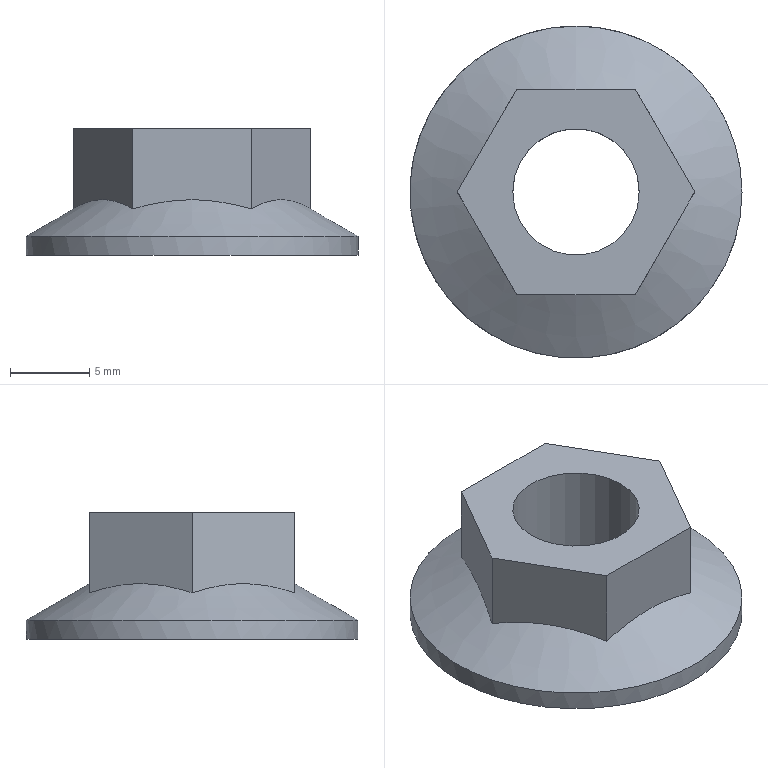Part | STEP file | 1_22 | 1 solid | 11 faces | box 21 x 21 x 8 mm | volume 1207 mm3 | plane 8 | cylinder 2 | cone 1 | commonest cylinder face diameters 8 x1 21 x1
STEP:
#1=CARTESIAN_POINT('',(0.,0.,0.));
#2=DIRECTION('',(0.,0.,1.));
#3=DIRECTION('',(1.,0.,0.));
#4=AXIS2_PLACEMENT_3D('',#1,#2,#3);
#5=CARTESIAN_POINT('',(3.753,6.5,2.929));
#6=VERTEX_POINT('',#5);
#7=CARTESIAN_POINT('',(0.,6.5,3.509));
#8=VERTEX_POINT('',#7);
#9=CARTESIAN_POINT('',(10.362,6.5,0.2));
#10=CARTESIAN_POINT('',(0.,6.5,5.268));
#11=CARTESIAN_POINT('',(-10.362,6.5,0.2));
#12=(BOUNDED_CURVE()B_SPLINE_CURVE(2,(#9,#10,#11),.UNSPECIFIED.,.F.,.F.)B_SPLINE_CURVE_WITH_KNOTS((3,3),(0.,2.176),.PIECEWISE_BEZIER_KNOTS.)CURVE()GEOMETRIC_REPRESENTATION_ITEM()RATIONAL_B_SPLINE_CURVE((1.,1.882,1.))REPRESENTATION_ITEM(''));
#13=CARTESIAN_POINT('',(0.,0.,6.262));
#14=DIRECTION('',(0.,0.,-1.));
#15=DIRECTION('',(0.,1.,0.));
#16=AXIS2_PLACEMENT_3D('',#13,#14,#15);
#17=CONICAL_SURFACE('',#16,1.732,1.047);
#18=CARTESIAN_POINT('',(0.5236,3.333));
#19=CARTESIAN_POINT('',(0.516,3.314));
#20=CARTESIAN_POINT('',(0.5008,3.278));
#21=CARTESIAN_POINT('',(0.4779,3.226));
#22=CARTESIAN_POINT('',(0.4548,3.177));
#23=CARTESIAN_POINT('',(0.4317,3.131));
#24=CARTESIAN_POINT('',(0.4084,3.088));
#25=CARTESIAN_POINT('',(0.3849,3.049));
#26=CARTESIAN_POINT('',(0.3614,3.011));
#27=CARTESIAN_POINT('',(0.3378,2.977));
#28=CARTESIAN_POINT('',(0.3141,2.945));
#29=CARTESIAN_POINT('',(0.2903,2.916));
#30=CARTESIAN_POINT('',(0.2664,2.89));
#31=CARTESIAN_POINT('',(0.2424,2.865));
#32=CARTESIAN_POINT('',(0.2184,2.844));
#33=CARTESIAN_POINT('',(0.1943,2.824));
#34=CARTESIAN_POINT('',(0.1701,2.807));
#35=CARTESIAN_POINT('',(0.1459,2.793));
#36=CARTESIAN_POINT('',(0.1217,2.78));
#37=CARTESIAN_POINT('',(0.09736,2.77));
#38=CARTESIAN_POINT('',(0.07305,2.762));
#39=CARTESIAN_POINT('',(0.04871,2.757));
#40=CARTESIAN_POINT('',(0.02436,2.754));
#41=CARTESIAN_POINT('',(0.00812,2.753));
#42=CARTESIAN_POINT('',(0.,2.753));
#43=B_SPLINE_CURVE_WITH_KNOTS('',3,(#18,#19,#20,#21,#22,#23,#24,#25,#26,#27,#28,#29,#30,#31,#32,#33,#34,#35,#36,#37,#38,#39,#40,#41,#42),.UNSPECIFIED.,.F.,.F.,(4,1,1,1,1,1,1,1,1,1,1,1,1,1,1,1,1,1,1,1,1,1,4),(0.5609,0.5848,0.6088,0.6327,0.6567,0.6806,0.7046,0.7285,0.7525,0.7764,0.8004,0.8243,0.8483,0.8722,0.8962,0.9201,0.9441,0.968,0.992,1.016,1.04,1.064,1.088),.QUASI_UNIFORM_KNOTS.);
#44=(GEOMETRIC_REPRESENTATION_CONTEXT(2)PARAMETRIC_REPRESENTATION_CONTEXT()REPRESENTATION_CONTEXT('',''));
#45=DEFINITIONAL_REPRESENTATION('',(#43),#44);
#46=PCURVE('',#17,#45);
#47=CARTESIAN_POINT('',(-4.128,6.5,8.254));
#48=DIRECTION('',(0.,1.,0.));
#49=DIRECTION('',(0.,0.,1.));
#50=AXIS2_PLACEMENT_3D('',#47,#48,#49);
#51=PLANE('',#50);
#52=CARTESIAN_POINT('',(-8.054,14.49));
#53=CARTESIAN_POINT('',(-2.986,4.128));
#54=CARTESIAN_POINT('',(-8.054,-6.234));
#55=(BOUNDED_CURVE()B_SPLINE_CURVE(2,(#52,#53,#54),.UNSPECIFIED.,.F.,.F.)B_SPLINE_CURVE_WITH_KNOTS((3,3),(0.,2.176),.PIECEWISE_BEZIER_KNOTS.)CURVE()GEOMETRIC_REPRESENTATION_ITEM()RATIONAL_B_SPLINE_CURVE((1.,1.882,1.))REPRESENTATION_ITEM(''));
#56=(GEOMETRIC_REPRESENTATION_CONTEXT(2)PARAMETRIC_REPRESENTATION_CONTEXT()REPRESENTATION_CONTEXT('',''));
#57=DEFINITIONAL_REPRESENTATION('',(#55),#56);
#58=PCURVE('',#51,#57);
#59=SURFACE_CURVE('',#12,(#46,#58),.PCURVE_S1.);
#60=EDGE_CURVE('',#6,#8,#59,.T.);
#61=ORIENTED_EDGE('',*,*,#60,.F.);
#62=CARTESIAN_POINT('',(7.506,0.,2.929));
#63=VERTEX_POINT('',#62);
#64=CARTESIAN_POINT('',(10.81,-5.724,0.2));
#65=CARTESIAN_POINT('',(5.629,3.25,5.268));
#66=CARTESIAN_POINT('',(0.4481,12.224,0.2));
#67=(BOUNDED_CURVE()B_SPLINE_CURVE(2,(#64,#65,#66),.UNSPECIFIED.,.F.,.F.)B_SPLINE_CURVE_WITH_KNOTS((3,3),(0.,2.176),.PIECEWISE_BEZIER_KNOTS.)CURVE()GEOMETRIC_REPRESENTATION_ITEM()RATIONAL_B_SPLINE_CURVE((1.,1.882,1.))REPRESENTATION_ITEM(''));
#68=CARTESIAN_POINT('',(1.571,3.333));
#69=CARTESIAN_POINT('',(1.556,3.295));
#70=CARTESIAN_POINT('',(1.525,3.224));
#71=CARTESIAN_POINT('',(1.479,3.13));
#72=CARTESIAN_POINT('',(1.432,3.047));
#73=CARTESIAN_POINT('',(1.385,2.976));
#74=CARTESIAN_POINT('',(1.338,2.915));
#75=CARTESIAN_POINT('',(1.29,2.864));
#76=CARTESIAN_POINT('',(1.241,2.823));
#77=CARTESIAN_POINT('',(1.193,2.792));
#78=CARTESIAN_POINT('',(1.145,2.769));
#79=CARTESIAN_POINT('',(1.096,2.756));
#80=CARTESIAN_POINT('',(1.047,2.751));
#81=CARTESIAN_POINT('',(0.9985,2.756));
#82=CARTESIAN_POINT('',(0.9498,2.769));
#83=CARTESIAN_POINT('',(0.9013,2.792));
#84=CARTESIAN_POINT('',(0.8529,2.823));
#85=CARTESIAN_POINT('',(0.8048,2.864));
#86=CARTESIAN_POINT('',(0.7569,2.915));
#87=CARTESIAN_POINT('',(0.7094,2.976));
#88=CARTESIAN_POINT('',(0.6622,3.047));
#89=CARTESIAN_POINT('',(0.6155,3.13));
#90=CARTESIAN_POINT('',(0.5692,3.224));
#91=CARTESIAN_POINT('',(0.5388,3.295));
#92=CARTESIAN_POINT('',(0.5236,3.333));
#93=B_SPLINE_CURVE_WITH_KNOTS('',3,(#68,#69,#70,#71,#72,#73,#74,#75,#76,#77,#78,#79,#80,#81,#82,#83,#84,#85,#86,#87,#88,#89,#90,#91,#92),.UNSPECIFIED.,.F.,.F.,(4,1,1,1,1,1,1,1,1,1,1,1,1,1,1,1,1,1,1,1,1,1,4),(0.5609,0.6088,0.6567,0.7046,0.7525,0.8004,0.8483,0.8962,0.9441,0.992,1.04,1.088,1.136,1.184,1.231,1.279,1.327,1.375,1.423,1.471,1.519,1.567,1.615),.QUASI_UNIFORM_KNOTS.);
#94=(GEOMETRIC_REPRESENTATION_CONTEXT(2)PARAMETRIC_REPRESENTATION_CONTEXT()REPRESENTATION_CONTEXT('',''));
#95=DEFINITIONAL_REPRESENTATION('',(#93),#94);
#96=PCURVE('',#17,#95);
#97=CARTESIAN_POINT('',(3.565,6.825,8.254));
#98=DIRECTION('',(0.866,0.5,0.));
#99=DIRECTION('',(0.,0.,-1.));
#100=AXIS2_PLACEMENT_3D('',#97,#98,#99);
#101=PLANE('',#100);
#102=CARTESIAN_POINT('',(8.054,-14.49));
#103=CARTESIAN_POINT('',(2.986,-4.128));
#104=CARTESIAN_POINT('',(8.054,6.234));
#105=(BOUNDED_CURVE()B_SPLINE_CURVE(2,(#102,#103,#104),.UNSPECIFIED.,.F.,.F.)B_SPLINE_CURVE_WITH_KNOTS((3,3),(0.,2.176),.PIECEWISE_BEZIER_KNOTS.)CURVE()GEOMETRIC_REPRESENTATION_ITEM()RATIONAL_B_SPLINE_CURVE((1.,1.882,1.))REPRESENTATION_ITEM(''));
#106=(GEOMETRIC_REPRESENTATION_CONTEXT(2)PARAMETRIC_REPRESENTATION_CONTEXT()REPRESENTATION_CONTEXT('',''));
#107=DEFINITIONAL_REPRESENTATION('',(#105),#106);
#108=PCURVE('',#101,#107);
#109=SURFACE_CURVE('',#67,(#96,#108),.PCURVE_S1.);
#110=EDGE_CURVE('',#63,#6,#109,.T.);
#111=ORIENTED_EDGE('',*,*,#110,.F.);
#112=CARTESIAN_POINT('',(3.753,-6.5,2.929));
#113=VERTEX_POINT('',#112);
#114=CARTESIAN_POINT('',(0.4481,-12.224,0.2));
#115=CARTESIAN_POINT('',(5.629,-3.25,5.268));
#116=CARTESIAN_POINT('',(10.81,5.724,0.2));
#117=(BOUNDED_CURVE()B_SPLINE_CURVE(2,(#114,#115,#116),.UNSPECIFIED.,.F.,.F.)B_SPLINE_CURVE_WITH_KNOTS((3,3),(0.,2.176),.PIECEWISE_BEZIER_KNOTS.)CURVE()GEOMETRIC_REPRESENTATION_ITEM()RATIONAL_B_SPLINE_CURVE((1.,1.882,1.))REPRESENTATION_ITEM(''));
#118=CARTESIAN_POINT('',(2.618,3.333));
#119=CARTESIAN_POINT('',(2.603,3.295));
#120=CARTESIAN_POINT('',(2.572,3.224));
#121=CARTESIAN_POINT('',(2.526,3.13));
#122=CARTESIAN_POINT('',(2.479,3.047));
#123=CARTESIAN_POINT('',(2.432,2.976));
#124=CARTESIAN_POINT('',(2.385,2.915));
#125=CARTESIAN_POINT('',(2.337,2.864));
#126=CARTESIAN_POINT('',(2.289,2.823));
#127=CARTESIAN_POINT('',(2.24,2.792));
#128=CARTESIAN_POINT('',(2.192,2.769));
#129=CARTESIAN_POINT('',(2.143,2.756));
#130=CARTESIAN_POINT('',(2.094,2.751));
#131=CARTESIAN_POINT('',(2.046,2.756));
#132=CARTESIAN_POINT('',(1.997,2.769));
#133=CARTESIAN_POINT('',(1.948,2.792));
#134=CARTESIAN_POINT('',(1.9,2.823));
#135=CARTESIAN_POINT('',(1.852,2.864));
#136=CARTESIAN_POINT('',(1.804,2.915));
#137=CARTESIAN_POINT('',(1.757,2.976));
#138=CARTESIAN_POINT('',(1.709,3.047));
#139=CARTESIAN_POINT('',(1.663,3.13));
#140=CARTESIAN_POINT('',(1.616,3.224));
#141=CARTESIAN_POINT('',(1.586,3.295));
#142=CARTESIAN_POINT('',(1.571,3.333));
#143=B_SPLINE_CURVE_WITH_KNOTS('',3,(#118,#119,#120,#121,#122,#123,#124,#125,#126,#127,#128,#129,#130,#131,#132,#133,#134,#135,#136,#137,#138,#139,#140,#141,#142),.UNSPECIFIED.,.F.,.F.,(4,1,1,1,1,1,1,1,1,1,1,1,1,1,1,1,1,1,1,1,1,1,4),(0.5609,0.6088,0.6567,0.7046,0.7525,0.8004,0.8483,0.8962,0.9441,0.992,1.04,1.088,1.136,1.184,1.231,1.279,1.327,1.375,1.423,1.471,1.519,1.567,1.615),.QUASI_UNIFORM_KNOTS.);
#144=(GEOMETRIC_REPRESENTATION_CONTEXT(2)PARAMETRIC_REPRESENTATION_CONTEXT()REPRESENTATION_CONTEXT('',''));
#145=DEFINITIONAL_REPRESENTATION('',(#143),#144);
#146=PCURVE('',#17,#145);
#147=CARTESIAN_POINT('',(7.693,0.325,8.254));
#148=DIRECTION('',(0.866,-0.5,0.));
#149=DIRECTION('',(0.,0.,-1.));
#150=AXIS2_PLACEMENT_3D('',#147,#148,#149);
#151=PLANE('',#150);
#152=CARTESIAN_POINT('',(8.054,-14.49));
#153=CARTESIAN_POINT('',(2.986,-4.128));
#154=CARTESIAN_POINT('',(8.054,6.234));
#155=(BOUNDED_CURVE()B_SPLINE_CURVE(2,(#152,#153,#154),.UNSPECIFIED.,.F.,.F.)B_SPLINE_CURVE_WITH_KNOTS((3,3),(0.,2.176),.PIECEWISE_BEZIER_KNOTS.)CURVE()GEOMETRIC_REPRESENTATION_ITEM()RATIONAL_B_SPLINE_CURVE((1.,1.882,1.))REPRESENTATION_ITEM(''));
#156=(GEOMETRIC_REPRESENTATION_CONTEXT(2)PARAMETRIC_REPRESENTATION_CONTEXT()REPRESENTATION_CONTEXT('',''));
#157=DEFINITIONAL_REPRESENTATION('',(#155),#156);
#158=PCURVE('',#151,#157);
#159=SURFACE_CURVE('',#117,(#146,#158),.PCURVE_S1.);
#160=EDGE_CURVE('',#113,#63,#159,.T.);
#161=ORIENTED_EDGE('',*,*,#160,.F.);
#162=CARTESIAN_POINT('',(0.,-6.5,3.509));
#163=VERTEX_POINT('',#162);
#164=CARTESIAN_POINT('',(-10.362,-6.5,0.2));
#165=CARTESIAN_POINT('',(0.,-6.5,5.268));
#166=CARTESIAN_POINT('',(10.362,-6.5,0.2));
#167=(BOUNDED_CURVE()B_SPLINE_CURVE(2,(#164,#165,#166),.UNSPECIFIED.,.F.,.F.)B_SPLINE_CURVE_WITH_KNOTS((3,3),(0.,2.176),.PIECEWISE_BEZIER_KNOTS.)CURVE()GEOMETRIC_REPRESENTATION_ITEM()RATIONAL_B_SPLINE_CURVE((1.,1.882,1.))REPRESENTATION_ITEM(''));
#168=CARTESIAN_POINT('',(3.142,2.753));
#169=CARTESIAN_POINT('',(3.133,2.753));
#170=CARTESIAN_POINT('',(3.117,2.754));
#171=CARTESIAN_POINT('',(3.093,2.757));
#172=CARTESIAN_POINT('',(3.069,2.762));
#173=CARTESIAN_POINT('',(3.044,2.77));
#174=CARTESIAN_POINT('',(3.02,2.78));
#175=CARTESIAN_POINT('',(2.996,2.793));
#176=CARTESIAN_POINT('',(2.971,2.807));
#177=CARTESIAN_POINT('',(2.947,2.824));
#178=CARTESIAN_POINT('',(2.923,2.844));
#179=CARTESIAN_POINT('',(2.899,2.865));
#180=CARTESIAN_POINT('',(2.875,2.89));
#181=CARTESIAN_POINT('',(2.851,2.916));
#182=CARTESIAN_POINT('',(2.828,2.945));
#183=CARTESIAN_POINT('',(2.804,2.977));
#184=CARTESIAN_POINT('',(2.78,3.011));
#185=CARTESIAN_POINT('',(2.757,3.049));
#186=CARTESIAN_POINT('',(2.733,3.088));
#187=CARTESIAN_POINT('',(2.71,3.131));
#188=CARTESIAN_POINT('',(2.687,3.177));
#189=CARTESIAN_POINT('',(2.664,3.226));
#190=CARTESIAN_POINT('',(2.641,3.278));
#191=CARTESIAN_POINT('',(2.626,3.314));
#192=CARTESIAN_POINT('',(2.618,3.333));
#193=B_SPLINE_CURVE_WITH_KNOTS('',3,(#168,#169,#170,#171,#172,#173,#174,#175,#176,#177,#178,#179,#180,#181,#182,#183,#184,#185,#186,#187,#188,#189,#190,#191,#192),.UNSPECIFIED.,.F.,.F.,(4,1,1,1,1,1,1,1,1,1,1,1,1,1,1,1,1,1,1,1,1,1,4),(1.088,1.112,1.136,1.16,1.184,1.208,1.231,1.255,1.279,1.303,1.327,1.351,1.375,1.399,1.423,1.447,1.471,1.495,1.519,1.543,1.567,1.591,1.615),.QUASI_UNIFORM_KNOTS.);
#194=(GEOMETRIC_REPRESENTATION_CONTEXT(2)PARAMETRIC_REPRESENTATION_CONTEXT()REPRESENTATION_CONTEXT('',''));
#195=DEFINITIONAL_REPRESENTATION('',(#193),#194);
#196=PCURVE('',#17,#195);
#197=CARTESIAN_POINT('',(4.128,-6.5,8.254));
#198=DIRECTION('',(0.,-1.,0.));
#199=DIRECTION('',(0.,0.,-1.));
#200=AXIS2_PLACEMENT_3D('',#197,#198,#199);
#201=PLANE('',#200);
#202=CARTESIAN_POINT('',(8.054,-14.49));
#203=CARTESIAN_POINT('',(2.986,-4.128));
#204=CARTESIAN_POINT('',(8.054,6.234));
#205=(BOUNDED_CURVE()B_SPLINE_CURVE(2,(#202,#203,#204),.UNSPECIFIED.,.F.,.F.)B_SPLINE_CURVE_WITH_KNOTS((3,3),(0.,2.176),.PIECEWISE_BEZIER_KNOTS.)CURVE()GEOMETRIC_REPRESENTATION_ITEM()RATIONAL_B_SPLINE_CURVE((1.,1.882,1.))REPRESENTATION_ITEM(''));
#206=(GEOMETRIC_REPRESENTATION_CONTEXT(2)PARAMETRIC_REPRESENTATION_CONTEXT()REPRESENTATION_CONTEXT('',''));
#207=DEFINITIONAL_REPRESENTATION('',(#205),#206);
#208=PCURVE('',#201,#207);
#209=SURFACE_CURVE('',#167,(#196,#208),.PCURVE_S1.);
#210=EDGE_CURVE('',#163,#113,#209,.T.);
#211=ORIENTED_EDGE('',*,*,#210,.F.);
#212=CARTESIAN_POINT('',(-3.753,-6.5,2.929));
#213=VERTEX_POINT('',#212);
#214=CARTESIAN_POINT('',(-10.362,-6.5,0.2));
#215=CARTESIAN_POINT('',(0.,-6.5,5.268));
#216=CARTESIAN_POINT('',(10.362,-6.5,0.2));
#217=(BOUNDED_CURVE()B_SPLINE_CURVE(2,(#214,#215,#216),.UNSPECIFIED.,.F.,.F.)B_SPLINE_CURVE_WITH_KNOTS((3,3),(0.,2.176),.PIECEWISE_BEZIER_KNOTS.)CURVE()GEOMETRIC_REPRESENTATION_ITEM()RATIONAL_B_SPLINE_CURVE((1.,1.882,1.))REPRESENTATION_ITEM(''));
#218=CARTESIAN_POINT('',(3.665,3.333));
#219=CARTESIAN_POINT('',(3.658,3.314));
#220=CARTESIAN_POINT('',(3.642,3.278));
#221=CARTESIAN_POINT('',(3.619,3.226));
#222=CARTESIAN_POINT('',(3.596,3.177));
#223=CARTESIAN_POINT('',(3.573,3.131));
#224=CARTESIAN_POINT('',(3.55,3.088));
#225=CARTESIAN_POINT('',(3.527,3.049));
#226=CARTESIAN_POINT('',(3.503,3.011));
#227=CARTESIAN_POINT('',(3.479,2.977));
#228=CARTESIAN_POINT('',(3.456,2.945));
#229=CARTESIAN_POINT('',(3.432,2.916));
#230=CARTESIAN_POINT('',(3.408,2.89));
#231=CARTESIAN_POINT('',(3.384,2.865));
#232=CARTESIAN_POINT('',(3.36,2.844));
#233=CARTESIAN_POINT('',(3.336,2.824));
#234=CARTESIAN_POINT('',(3.312,2.807));
#235=CARTESIAN_POINT('',(3.287,2.793));
#236=CARTESIAN_POINT('',(3.263,2.78));
#237=CARTESIAN_POINT('',(3.239,2.77));
#238=CARTESIAN_POINT('',(3.215,2.762));
#239=CARTESIAN_POINT('',(3.19,2.757));
#240=CARTESIAN_POINT('',(3.166,2.754));
#241=CARTESIAN_POINT('',(3.15,2.753));
#242=CARTESIAN_POINT('',(3.142,2.753));
#243=B_SPLINE_CURVE_WITH_KNOTS('',3,(#218,#219,#220,#221,#222,#223,#224,#225,#226,#227,#228,#229,#230,#231,#232,#233,#234,#235,#236,#237,#238,#239,#240,#241,#242),.UNSPECIFIED.,.F.,.F.,(4,1,1,1,1,1,1,1,1,1,1,1,1,1,1,1,1,1,1,1,1,1,4),(0.5609,0.5848,0.6088,0.6327,0.6567,0.6806,0.7046,0.7285,0.7525,0.7764,0.8004,0.8243,0.8483,0.8722,0.8962,0.9201,0.9441,0.968,0.992,1.016,1.04,1.064,1.088),.QUASI_UNIFORM_KNOTS.);
#244=(GEOMETRIC_REPRESENTATION_CONTEXT(2)PARAMETRIC_REPRESENTATION_CONTEXT()REPRESENTATION_CONTEXT('',''));
#245=DEFINITIONAL_REPRESENTATION('',(#243),#244);
#246=PCURVE('',#17,#245);
#247=CARTESIAN_POINT('',(8.054,-14.49));
#248=CARTESIAN_POINT('',(2.986,-4.128));
#249=CARTESIAN_POINT('',(8.054,6.234));
#250=(BOUNDED_CURVE()B_SPLINE_CURVE(2,(#247,#248,#249),.UNSPECIFIED.,.F.,.F.)B_SPLINE_CURVE_WITH_KNOTS((3,3),(0.,2.176),.PIECEWISE_BEZIER_KNOTS.)CURVE()GEOMETRIC_REPRESENTATION_ITEM()RATIONAL_B_SPLINE_CURVE((1.,1.882,1.))REPRESENTATION_ITEM(''));
#251=(GEOMETRIC_REPRESENTATION_CONTEXT(2)PARAMETRIC_REPRESENTATION_CONTEXT()REPRESENTATION_CONTEXT('',''));
#252=DEFINITIONAL_REPRESENTATION('',(#250),#251);
#253=PCURVE('',#201,#252);
#254=SURFACE_CURVE('',#217,(#246,#253),.PCURVE_S1.);
#255=EDGE_CURVE('',#213,#163,#254,.T.);
#256=ORIENTED_EDGE('',*,*,#255,.F.);
#257=CARTESIAN_POINT('',(-7.506,0.,2.929));
#258=VERTEX_POINT('',#257);
#259=CARTESIAN_POINT('',(-10.81,5.724,0.2));
#260=CARTESIAN_POINT('',(-5.629,-3.25,5.268));
#261=CARTESIAN_POINT('',(-0.4481,-12.224,0.2));
#262=(BOUNDED_CURVE()B_SPLINE_CURVE(2,(#259,#260,#261),.UNSPECIFIED.,.F.,.F.)B_SPLINE_CURVE_WITH_KNOTS((3,3),(0.,2.176),.PIECEWISE_BEZIER_KNOTS.)CURVE()GEOMETRIC_REPRESENTATION_ITEM()RATIONAL_B_SPLINE_CURVE((1.,1.882,1.))REPRESENTATION_ITEM(''));
#263=CARTESIAN_POINT('',(4.712,3.333));
#264=CARTESIAN_POINT('',(4.697,3.295));
#265=CARTESIAN_POINT('',(4.667,3.224));
#266=CARTESIAN_POINT('',(4.621,3.13));
#267=CARTESIAN_POINT('',(4.574,3.047));
#268=CARTESIAN_POINT('',(4.527,2.976));
#269=CARTESIAN_POINT('',(4.479,2.915));
#270=CARTESIAN_POINT('',(4.431,2.864));
#271=CARTESIAN_POINT('',(4.383,2.823));
#272=CARTESIAN_POINT('',(4.335,2.792));
#273=CARTESIAN_POINT('',(4.286,2.769));
#274=CARTESIAN_POINT('',(4.238,2.756));
#275=CARTESIAN_POINT('',(4.189,2.751));
#276=CARTESIAN_POINT('',(4.14,2.756));
#277=CARTESIAN_POINT('',(4.091,2.769));
#278=CARTESIAN_POINT('',(4.043,2.792));
#279=CARTESIAN_POINT('',(3.994,2.823));
#280=CARTESIAN_POINT('',(3.946,2.864));
#281=CARTESIAN_POINT('',(3.898,2.915));
#282=CARTESIAN_POINT('',(3.851,2.976));
#283=CARTESIAN_POINT('',(3.804,3.047));
#284=CARTESIAN_POINT('',(3.757,3.13));
#285=CARTESIAN_POINT('',(3.711,3.224));
#286=CARTESIAN_POINT('',(3.68,3.295));
#287=CARTESIAN_POINT('',(3.665,3.333));
#288=B_SPLINE_CURVE_WITH_KNOTS('',3,(#263,#264,#265,#266,#267,#268,#269,#270,#271,#272,#273,#274,#275,#276,#277,#278,#279,#280,#281,#282,#283,#284,#285,#286,#287),.UNSPECIFIED.,.F.,.F.,(4,1,1,1,1,1,1,1,1,1,1,1,1,1,1,1,1,1,1,1,1,1,4),(0.5609,0.6088,0.6567,0.7046,0.7525,0.8004,0.8483,0.8962,0.9441,0.992,1.04,1.088,1.136,1.184,1.231,1.279,1.327,1.375,1.423,1.471,1.519,1.567,1.615),.QUASI_UNIFORM_KNOTS.);
#289=(GEOMETRIC_REPRESENTATION_CONTEXT(2)PARAMETRIC_REPRESENTATION_CONTEXT()REPRESENTATION_CONTEXT('',''));
#290=DEFINITIONAL_REPRESENTATION('',(#288),#289);
#291=PCURVE('',#17,#290);
#292=CARTESIAN_POINT('',(-3.565,-6.825,8.254));
#293=DIRECTION('',(-0.866,-0.5,0.));
#294=DIRECTION('',(0.,0.,1.));
#295=AXIS2_PLACEMENT_3D('',#292,#293,#294);
#296=PLANE('',#295);
#297=CARTESIAN_POINT('',(-8.054,14.49));
#298=CARTESIAN_POINT('',(-2.986,4.128));
#299=CARTESIAN_POINT('',(-8.054,-6.234));
#300=(BOUNDED_CURVE()B_SPLINE_CURVE(2,(#297,#298,#299),.UNSPECIFIED.,.F.,.F.)B_SPLINE_CURVE_WITH_KNOTS((3,3),(0.,2.176),.PIECEWISE_BEZIER_KNOTS.)CURVE()GEOMETRIC_REPRESENTATION_ITEM()RATIONAL_B_SPLINE_CURVE((1.,1.882,1.))REPRESENTATION_ITEM(''));
#301=(GEOMETRIC_REPRESENTATION_CONTEXT(2)PARAMETRIC_REPRESENTATION_CONTEXT()REPRESENTATION_CONTEXT('',''));
#302=DEFINITIONAL_REPRESENTATION('',(#300),#301);
#303=PCURVE('',#296,#302);
#304=SURFACE_CURVE('',#262,(#291,#303),.PCURVE_S1.);
#305=EDGE_CURVE('',#258,#213,#304,.T.);
#306=ORIENTED_EDGE('',*,*,#305,.F.);
#307=CARTESIAN_POINT('',(-3.753,6.5,2.929));
#308=VERTEX_POINT('',#307);
#309=CARTESIAN_POINT('',(-0.4481,12.224,0.2));
#310=CARTESIAN_POINT('',(-5.629,3.25,5.268));
#311=CARTESIAN_POINT('',(-10.81,-5.724,0.2));
#312=(BOUNDED_CURVE()B_SPLINE_CURVE(2,(#309,#310,#311),.UNSPECIFIED.,.F.,.F.)B_SPLINE_CURVE_WITH_KNOTS((3,3),(0.,2.176),.PIECEWISE_BEZIER_KNOTS.)CURVE()GEOMETRIC_REPRESENTATION_ITEM()RATIONAL_B_SPLINE_CURVE((1.,1.882,1.))REPRESENTATION_ITEM(''));
#313=CARTESIAN_POINT('',(5.76,3.333));
#314=CARTESIAN_POINT('',(5.744,3.295));
#315=CARTESIAN_POINT('',(5.714,3.224));
#316=CARTESIAN_POINT('',(5.668,3.13));
#317=CARTESIAN_POINT('',(5.621,3.047));
#318=CARTESIAN_POINT('',(5.574,2.976));
#319=CARTESIAN_POINT('',(5.526,2.915));
#320=CARTESIAN_POINT('',(5.478,2.864));
#321=CARTESIAN_POINT('',(5.43,2.823));
#322=CARTESIAN_POINT('',(5.382,2.792));
#323=CARTESIAN_POINT('',(5.333,2.769));
#324=CARTESIAN_POINT('',(5.285,2.756));
#325=CARTESIAN_POINT('',(5.236,2.751));
#326=CARTESIAN_POINT('',(5.187,2.756));
#327=CARTESIAN_POINT('',(5.139,2.769));
#328=CARTESIAN_POINT('',(5.09,2.792));
#329=CARTESIAN_POINT('',(5.042,2.823));
#330=CARTESIAN_POINT('',(4.994,2.864));
#331=CARTESIAN_POINT('',(4.946,2.915));
#332=CARTESIAN_POINT('',(4.898,2.976));
#333=CARTESIAN_POINT('',(4.851,3.047));
#334=CARTESIAN_POINT('',(4.804,3.13));
#335=CARTESIAN_POINT('',(4.758,3.224));
#336=CARTESIAN_POINT('',(4.728,3.295));
#337=CARTESIAN_POINT('',(4.712,3.333));
#338=B_SPLINE_CURVE_WITH_KNOTS('',3,(#313,#314,#315,#316,#317,#318,#319,#320,#321,#322,#323,#324,#325,#326,#327,#328,#329,#330,#331,#332,#333,#334,#335,#336,#337),.UNSPECIFIED.,.F.,.F.,(4,1,1,1,1,1,1,1,1,1,1,1,1,1,1,1,1,1,1,1,1,1,4),(0.5609,0.6088,0.6567,0.7046,0.7525,0.8004,0.8483,0.8962,0.9441,0.992,1.04,1.088,1.136,1.184,1.231,1.279,1.327,1.375,1.423,1.471,1.519,1.567,1.615),.QUASI_UNIFORM_KNOTS.);
#339=(GEOMETRIC_REPRESENTATION_CONTEXT(2)PARAMETRIC_REPRESENTATION_CONTEXT()REPRESENTATION_CONTEXT('',''));
#340=DEFINITIONAL_REPRESENTATION('',(#338),#339);
#341=PCURVE('',#17,#340);
#342=CARTESIAN_POINT('',(-7.693,-0.325,8.254));
#343=DIRECTION('',(-0.866,0.5,0.));
#344=DIRECTION('',(0.,0.,1.));
#345=AXIS2_PLACEMENT_3D('',#342,#343,#344);
#346=PLANE('',#345);
#347=CARTESIAN_POINT('',(-8.054,14.49));
#348=CARTESIAN_POINT('',(-2.986,4.128));
#349=CARTESIAN_POINT('',(-8.054,-6.234));
#350=(BOUNDED_CURVE()B_SPLINE_CURVE(2,(#347,#348,#349),.UNSPECIFIED.,.F.,.F.)B_SPLINE_CURVE_WITH_KNOTS((3,3),(0.,2.176),.PIECEWISE_BEZIER_KNOTS.)CURVE()GEOMETRIC_REPRESENTATION_ITEM()RATIONAL_B_SPLINE_CURVE((1.,1.882,1.))REPRESENTATION_ITEM(''));
#351=(GEOMETRIC_REPRESENTATION_CONTEXT(2)PARAMETRIC_REPRESENTATION_CONTEXT()REPRESENTATION_CONTEXT('',''));
#352=DEFINITIONAL_REPRESENTATION('',(#350),#351);
#353=PCURVE('',#346,#352);
#354=SURFACE_CURVE('',#312,(#341,#353),.PCURVE_S1.);
#355=EDGE_CURVE('',#308,#258,#354,.T.);
#356=ORIENTED_EDGE('',*,*,#355,.F.);
#357=CARTESIAN_POINT('',(10.362,6.5,0.2));
#358=CARTESIAN_POINT('',(0.,6.5,5.268));
#359=CARTESIAN_POINT('',(-10.362,6.5,0.2));
#360=(BOUNDED_CURVE()B_SPLINE_CURVE(2,(#357,#358,#359),.UNSPECIFIED.,.F.,.F.)B_SPLINE_CURVE_WITH_KNOTS((3,3),(0.,2.176),.PIECEWISE_BEZIER_KNOTS.)CURVE()GEOMETRIC_REPRESENTATION_ITEM()RATIONAL_B_SPLINE_CURVE((1.,1.882,1.))REPRESENTATION_ITEM(''));
#361=CARTESIAN_POINT('',(6.283,2.753));
#362=CARTESIAN_POINT('',(6.275,2.753));
#363=CARTESIAN_POINT('',(6.259,2.754));
#364=CARTESIAN_POINT('',(6.234,2.757));
#365=CARTESIAN_POINT('',(6.21,2.762));
#366=CARTESIAN_POINT('',(6.186,2.77));
#367=CARTESIAN_POINT('',(6.162,2.78));
#368=CARTESIAN_POINT('',(6.137,2.793));
#369=CARTESIAN_POINT('',(6.113,2.807));
#370=CARTESIAN_POINT('',(6.089,2.824));
#371=CARTESIAN_POINT('',(6.065,2.844));
#372=CARTESIAN_POINT('',(6.041,2.865));
#373=CARTESIAN_POINT('',(6.017,2.89));
#374=CARTESIAN_POINT('',(5.993,2.916));
#375=CARTESIAN_POINT('',(5.969,2.945));
#376=CARTESIAN_POINT('',(5.945,2.977));
#377=CARTESIAN_POINT('',(5.922,3.011));
#378=CARTESIAN_POINT('',(5.898,3.049));
#379=CARTESIAN_POINT('',(5.875,3.088));
#380=CARTESIAN_POINT('',(5.852,3.131));
#381=CARTESIAN_POINT('',(5.828,3.177));
#382=CARTESIAN_POINT('',(5.805,3.226));
#383=CARTESIAN_POINT('',(5.782,3.278));
#384=CARTESIAN_POINT('',(5.767,3.314));
#385=CARTESIAN_POINT('',(5.76,3.333));
#386=B_SPLINE_CURVE_WITH_KNOTS('',3,(#361,#362,#363,#364,#365,#366,#367,#368,#369,#370,#371,#372,#373,#374,#375,#376,#377,#378,#379,#380,#381,#382,#383,#384,#385),.UNSPECIFIED.,.F.,.F.,(4,1,1,1,1,1,1,1,1,1,1,1,1,1,1,1,1,1,1,1,1,1,4),(1.088,1.112,1.136,1.16,1.184,1.208,1.231,1.255,1.279,1.303,1.327,1.351,1.375,1.399,1.423,1.447,1.471,1.495,1.519,1.543,1.567,1.591,1.615),.QUASI_UNIFORM_KNOTS.);
#387=(GEOMETRIC_REPRESENTATION_CONTEXT(2)PARAMETRIC_REPRESENTATION_CONTEXT()REPRESENTATION_CONTEXT('',''));
#388=DEFINITIONAL_REPRESENTATION('',(#386),#387);
#389=PCURVE('',#17,#388);
#390=CARTESIAN_POINT('',(-8.054,14.49));
#391=CARTESIAN_POINT('',(-2.986,4.128));
#392=CARTESIAN_POINT('',(-8.054,-6.234));
#393=(BOUNDED_CURVE()B_SPLINE_CURVE(2,(#390,#391,#392),.UNSPECIFIED.,.F.,.F.)B_SPLINE_CURVE_WITH_KNOTS((3,3),(0.,2.176),.PIECEWISE_BEZIER_KNOTS.)CURVE()GEOMETRIC_REPRESENTATION_ITEM()RATIONAL_B_SPLINE_CURVE((1.,1.882,1.))REPRESENTATION_ITEM(''));
#394=(GEOMETRIC_REPRESENTATION_CONTEXT(2)PARAMETRIC_REPRESENTATION_CONTEXT()REPRESENTATION_CONTEXT('',''));
#395=DEFINITIONAL_REPRESENTATION('',(#393),#394);
#396=PCURVE('',#51,#395);
#397=SURFACE_CURVE('',#360,(#389,#396),.PCURVE_S1.);
#398=EDGE_CURVE('',#8,#308,#397,.T.);
#399=ORIENTED_EDGE('',*,*,#398,.F.);
#400=CARTESIAN_POINT('',(0.,10.5,1.2));
#401=VERTEX_POINT('',#400);
#402=CARTESIAN_POINT('',(0.,6.5,3.509));
#403=CARTESIAN_POINT('',(0.,10.5,1.2));
#404=B_SPLINE_CURVE_WITH_KNOTS('',1,(#402,#403),.UNSPECIFIED.,.F.,.F.,(2,2),(5.506,10.124),.PIECEWISE_BEZIER_KNOTS.);
#405=CARTESIAN_POINT('',(6.283,0.));
#406=DIRECTION('',(0.,1.));
#407=VECTOR('',#406,1.);
#408=LINE('',#405,#407);
#409=(GEOMETRIC_REPRESENTATION_CONTEXT(2)PARAMETRIC_REPRESENTATION_CONTEXT()REPRESENTATION_CONTEXT('',''));
#410=DEFINITIONAL_REPRESENTATION('',(#408),#409);
#411=PCURVE('',#17,#410);
#412=CARTESIAN_POINT('',(0.,0.));
#413=DIRECTION('',(0.,1.));
#414=VECTOR('',#413,1.);
#415=LINE('',#412,#414);
#416=(GEOMETRIC_REPRESENTATION_CONTEXT(2)PARAMETRIC_REPRESENTATION_CONTEXT()REPRESENTATION_CONTEXT('',''));
#417=DEFINITIONAL_REPRESENTATION('',(#415),#416);
#418=PCURVE('',#17,#417);
#419=SEAM_CURVE('',#404,(#411,#418),.PCURVE_S1.);
#420=EDGE_CURVE('',#8,#401,#419,.T.);
#421=ORIENTED_EDGE('',*,*,#420,.T.);
#422=CARTESIAN_POINT('',(10.5,0.,1.2));
#423=VERTEX_POINT('',#422);
#424=CARTESIAN_POINT('',(0.,0.,1.2));
#425=DIRECTION('',(0.,0.,-1.));
#426=DIRECTION('',(1.,0.,0.));
#427=AXIS2_PLACEMENT_3D('',#424,#425,#426);
#428=CIRCLE('',#427,10.5);
#429=CARTESIAN_POINT('',(-4.712,5.062));
#430=DIRECTION('',(1.,0.));
#431=VECTOR('',#430,1.);
#432=LINE('',#429,#431);
#433=(GEOMETRIC_REPRESENTATION_CONTEXT(2)PARAMETRIC_REPRESENTATION_CONTEXT()REPRESENTATION_CONTEXT('',''));
#434=DEFINITIONAL_REPRESENTATION('',(#432),#433);
#435=PCURVE('',#17,#434);
#436=CARTESIAN_POINT('',(0.,0.,8.4));
#437=DIRECTION('',(0.,0.,-1.));
#438=DIRECTION('',(1.,0.,0.));
#439=AXIS2_PLACEMENT_3D('',#436,#437,#438);
#440=CYLINDRICAL_SURFACE('',#439,10.5);
#441=CARTESIAN_POINT('',(-6.283,7.2));
#442=DIRECTION('',(1.,0.));
#443=VECTOR('',#442,1.);
#444=LINE('',#441,#443);
#445=(GEOMETRIC_REPRESENTATION_CONTEXT(2)PARAMETRIC_REPRESENTATION_CONTEXT()REPRESENTATION_CONTEXT('',''));
#446=DEFINITIONAL_REPRESENTATION('',(#444),#445);
#447=PCURVE('',#440,#446);
#448=SURFACE_CURVE('',#428,(#435,#447),.PCURVE_S1.);
#449=EDGE_CURVE('',#423,#401,#448,.T.);
#450=ORIENTED_EDGE('',*,*,#449,.F.);
#451=CARTESIAN_POINT('',(0.,0.,1.2));
#452=DIRECTION('',(0.,0.,-1.));
#453=DIRECTION('',(1.,0.,0.));
#454=AXIS2_PLACEMENT_3D('',#451,#452,#453);
#455=CIRCLE('',#454,10.5);
#456=CARTESIAN_POINT('',(-4.712,5.062));
#457=DIRECTION('',(1.,0.));
#458=VECTOR('',#457,1.);
#459=LINE('',#456,#458);
#460=(GEOMETRIC_REPRESENTATION_CONTEXT(2)PARAMETRIC_REPRESENTATION_CONTEXT()REPRESENTATION_CONTEXT('',''));
#461=DEFINITIONAL_REPRESENTATION('',(#459),#460);
#462=PCURVE('',#17,#461);
#463=CARTESIAN_POINT('',(0.,7.2));
#464=DIRECTION('',(1.,0.));
#465=VECTOR('',#464,1.);
#466=LINE('',#463,#465);
#467=(GEOMETRIC_REPRESENTATION_CONTEXT(2)PARAMETRIC_REPRESENTATION_CONTEXT()REPRESENTATION_CONTEXT('',''));
#468=DEFINITIONAL_REPRESENTATION('',(#466),#467);
#469=PCURVE('',#440,#468);
#470=SURFACE_CURVE('',#455,(#462,#469),.PCURVE_S1.);
#471=EDGE_CURVE('',#401,#423,#470,.T.);
#472=ORIENTED_EDGE('',*,*,#471,.F.);
#473=ORIENTED_EDGE('',*,*,#420,.F.);
#474=EDGE_LOOP('',(#61,#111,#161,#211,#256,#306,#356,#399,#421,#450,#472,#473));
#475=FACE_BOUND('',#474,.T.);
#476=ADVANCED_FACE('',(#475),#17,.T.);
#477=ORIENTED_EDGE('',*,*,#471,.T.);
#478=CARTESIAN_POINT('',(10.5,0.,0.));
#479=VERTEX_POINT('',#478);
#480=CARTESIAN_POINT('',(10.5,0.,1.2));
#481=CARTESIAN_POINT('',(10.5,0.,0.));
#482=B_SPLINE_CURVE_WITH_KNOTS('',1,(#480,#481),.UNSPECIFIED.,.F.,.F.,(2,2),(7.2,8.4),.PIECEWISE_BEZIER_KNOTS.);
#483=CARTESIAN_POINT('',(6.283,0.));
#484=DIRECTION('',(0.,1.));
#485=VECTOR('',#484,1.);
#486=LINE('',#483,#485);
#487=(GEOMETRIC_REPRESENTATION_CONTEXT(2)PARAMETRIC_REPRESENTATION_CONTEXT()REPRESENTATION_CONTEXT('',''));
#488=DEFINITIONAL_REPRESENTATION('',(#486),#487);
#489=PCURVE('',#440,#488);
#490=CARTESIAN_POINT('',(0.,0.));
#491=DIRECTION('',(0.,1.));
#492=VECTOR('',#491,1.);
#493=LINE('',#490,#492);
#494=(GEOMETRIC_REPRESENTATION_CONTEXT(2)PARAMETRIC_REPRESENTATION_CONTEXT()REPRESENTATION_CONTEXT('',''));
#495=DEFINITIONAL_REPRESENTATION('',(#493),#494);
#496=PCURVE('',#440,#495);
#497=SEAM_CURVE('',#482,(#489,#496),.PCURVE_S1.);
#498=EDGE_CURVE('',#423,#479,#497,.T.);
#499=ORIENTED_EDGE('',*,*,#498,.T.);
#500=CARTESIAN_POINT('',(0.,0.,0.));
#501=DIRECTION('',(0.,0.,-1.));
#502=DIRECTION('',(-1.,0.,0.));
#503=AXIS2_PLACEMENT_3D('',#500,#501,#502);
#504=CIRCLE('',#503,10.5);
#505=CARTESIAN_POINT('',(-3.142,8.4));
#506=DIRECTION('',(1.,0.));
#507=VECTOR('',#506,1.);
#508=LINE('',#505,#507);
#509=(GEOMETRIC_REPRESENTATION_CONTEXT(2)PARAMETRIC_REPRESENTATION_CONTEXT()REPRESENTATION_CONTEXT('',''));
#510=DEFINITIONAL_REPRESENTATION('',(#508),#509);
#511=PCURVE('',#440,#510);
#512=CARTESIAN_POINT('',(11.55,-11.55,0.));
#513=DIRECTION('',(0.,0.,-1.));
#514=DIRECTION('',(-1.,0.,0.));
#515=AXIS2_PLACEMENT_3D('',#512,#513,#514);
#516=PLANE('',#515);
#517=CARTESIAN_POINT('',(11.55,11.55));
#518=DIRECTION('',(1.,0.));
#519=AXIS2_PLACEMENT_2D('',#517,#518);
#520=CIRCLE('',#519,10.5);
#521=(GEOMETRIC_REPRESENTATION_CONTEXT(2)PARAMETRIC_REPRESENTATION_CONTEXT()REPRESENTATION_CONTEXT('',''));
#522=DEFINITIONAL_REPRESENTATION('',(#520),#521);
#523=PCURVE('',#516,#522);
#524=SURFACE_CURVE('',#504,(#511,#523),.PCURVE_S1.);
#525=EDGE_CURVE('',#479,#479,#524,.T.);
#526=ORIENTED_EDGE('',*,*,#525,.F.);
#527=ORIENTED_EDGE('',*,*,#498,.F.);
#528=ORIENTED_EDGE('',*,*,#449,.T.);
#529=EDGE_LOOP('',(#477,#499,#526,#527,#528));
#530=FACE_BOUND('',#529,.T.);
#531=ADVANCED_FACE('',(#530),#440,.T.);
#532=CARTESIAN_POINT('',(3.753,-6.5,8.));
#533=VERTEX_POINT('',#532);
#534=CARTESIAN_POINT('',(3.753,-6.5,8.));
#535=DIRECTION('',(0.,0.,-1.));
#536=VECTOR('',#535,1.);
#537=LINE('',#534,#536);
#538=CARTESIAN_POINT('',(0.2536,-7.881));
#539=DIRECTION('',(1.,0.));
#540=VECTOR('',#539,1.);
#541=LINE('',#538,#540);
#542=(GEOMETRIC_REPRESENTATION_CONTEXT(2)PARAMETRIC_REPRESENTATION_CONTEXT()REPRESENTATION_CONTEXT('',''));
#543=DEFINITIONAL_REPRESENTATION('',(#541),#542);
#544=PCURVE('',#151,#543);
#545=CARTESIAN_POINT('',(0.2536,-0.3753));
#546=DIRECTION('',(1.,0.));
#547=VECTOR('',#546,1.);
#548=LINE('',#545,#547);
#549=(GEOMETRIC_REPRESENTATION_CONTEXT(2)PARAMETRIC_REPRESENTATION_CONTEXT()REPRESENTATION_CONTEXT('',''));
#550=DEFINITIONAL_REPRESENTATION('',(#548),#549);
#551=PCURVE('',#201,#550);
#552=SURFACE_CURVE('',#537,(#544,#551),.PCURVE_S1.);
#553=EDGE_CURVE('',#533,#113,#552,.T.);
#554=ORIENTED_EDGE('',*,*,#553,.T.);
#555=ORIENTED_EDGE('',*,*,#160,.T.);
#556=CARTESIAN_POINT('',(7.506,0.,8.));
#557=VERTEX_POINT('',#556);
#558=CARTESIAN_POINT('',(7.506,-0.000000001,8.));
#559=DIRECTION('',(0.,0.,-1.));
#560=VECTOR('',#559,1.);
#561=LINE('',#558,#560);
#562=CARTESIAN_POINT('',(0.2536,-0.3753));
#563=DIRECTION('',(1.,0.));
#564=VECTOR('',#563,1.);
#565=LINE('',#562,#564);
#566=(GEOMETRIC_REPRESENTATION_CONTEXT(2)PARAMETRIC_REPRESENTATION_CONTEXT()REPRESENTATION_CONTEXT('',''));
#567=DEFINITIONAL_REPRESENTATION('',(#565),#566);
#568=PCURVE('',#151,#567);
#569=CARTESIAN_POINT('',(0.2536,-7.881));
#570=DIRECTION('',(1.,0.));
#571=VECTOR('',#570,1.);
#572=LINE('',#569,#571);
#573=(GEOMETRIC_REPRESENTATION_CONTEXT(2)PARAMETRIC_REPRESENTATION_CONTEXT()REPRESENTATION_CONTEXT('',''));
#574=DEFINITIONAL_REPRESENTATION('',(#572),#573);
#575=PCURVE('',#101,#574);
#576=SURFACE_CURVE('',#561,(#568,#575),.PCURVE_S1.);
#577=EDGE_CURVE('',#557,#63,#576,.T.);
#578=ORIENTED_EDGE('',*,*,#577,.F.);
#579=CARTESIAN_POINT('',(7.506,0.,8.));
#580=DIRECTION('',(-0.5,-0.866,0.));
#581=VECTOR('',#580,1.);
#582=LINE('',#579,#581);
#583=CARTESIAN_POINT('',(0.2536,-0.3753));
#584=DIRECTION('',(0.,-1.));
#585=VECTOR('',#584,1.);
#586=LINE('',#583,#585);
#587=(GEOMETRIC_REPRESENTATION_CONTEXT(2)PARAMETRIC_REPRESENTATION_CONTEXT()REPRESENTATION_CONTEXT('',''));
#588=DEFINITIONAL_REPRESENTATION('',(#586),#587);
#589=PCURVE('',#151,#588);
#590=CARTESIAN_POINT('',(8.256,-7.15,8.));
#591=DIRECTION('',(0.,0.,-1.));
#592=DIRECTION('',(-1.,0.,0.));
#593=AXIS2_PLACEMENT_3D('',#590,#591,#592);
#594=PLANE('',#593);
#595=CARTESIAN_POINT('',(0.7506,7.15));
#596=DIRECTION('',(0.5,-0.866));
#597=VECTOR('',#596,1.);
#598=LINE('',#595,#597);
#599=(GEOMETRIC_REPRESENTATION_CONTEXT(2)PARAMETRIC_REPRESENTATION_CONTEXT()REPRESENTATION_CONTEXT('',''));
#600=DEFINITIONAL_REPRESENTATION('',(#598),#599);
#601=PCURVE('',#594,#600);
#602=SURFACE_CURVE('',#582,(#589,#601),.PCURVE_S1.);
#603=EDGE_CURVE('',#557,#533,#602,.T.);
#604=ORIENTED_EDGE('',*,*,#603,.T.);
#605=EDGE_LOOP('',(#554,#555,#578,#604));
#606=FACE_BOUND('',#605,.T.);
#607=ADVANCED_FACE('',(#606),#151,.T.);
#608=CARTESIAN_POINT('',(-3.753,-6.5,8.));
#609=VERTEX_POINT('',#608);
#610=CARTESIAN_POINT('',(-3.753,-6.5,8.));
#611=DIRECTION('',(0.,0.,-1.));
#612=VECTOR('',#611,1.);
#613=LINE('',#610,#612);
#614=CARTESIAN_POINT('',(0.2536,-7.881));
#615=DIRECTION('',(1.,0.));
#616=VECTOR('',#615,1.);
#617=LINE('',#614,#616);
#618=(GEOMETRIC_REPRESENTATION_CONTEXT(2)PARAMETRIC_REPRESENTATION_CONTEXT()REPRESENTATION_CONTEXT('',''));
#619=DEFINITIONAL_REPRESENTATION('',(#617),#618);
#620=PCURVE('',#201,#619);
#621=CARTESIAN_POINT('',(-0.2536,0.3753));
#622=DIRECTION('',(-1.,0.));
#623=VECTOR('',#622,1.);
#624=LINE('',#621,#623);
#625=(GEOMETRIC_REPRESENTATION_CONTEXT(2)PARAMETRIC_REPRESENTATION_CONTEXT()REPRESENTATION_CONTEXT('',''));
#626=DEFINITIONAL_REPRESENTATION('',(#624),#625);
#627=PCURVE('',#296,#626);
#628=SURFACE_CURVE('',#613,(#620,#627),.PCURVE_S1.);
#629=EDGE_CURVE('',#609,#213,#628,.T.);
#630=ORIENTED_EDGE('',*,*,#629,.T.);
#631=ORIENTED_EDGE('',*,*,#255,.T.);
#632=ORIENTED_EDGE('',*,*,#210,.T.);
#633=ORIENTED_EDGE('',*,*,#553,.F.);
#634=CARTESIAN_POINT('',(3.753,-6.5,8.));
#635=DIRECTION('',(-1.,0.,0.));
#636=VECTOR('',#635,1.);
#637=LINE('',#634,#636);
#638=CARTESIAN_POINT('',(0.2536,-0.3753));
#639=DIRECTION('',(0.,-1.));
#640=VECTOR('',#639,1.);
#641=LINE('',#638,#640);
#642=(GEOMETRIC_REPRESENTATION_CONTEXT(2)PARAMETRIC_REPRESENTATION_CONTEXT()REPRESENTATION_CONTEXT('',''));
#643=DEFINITIONAL_REPRESENTATION('',(#641),#642);
#644=PCURVE('',#201,#643);
#645=CARTESIAN_POINT('',(4.503,0.65));
#646=DIRECTION('',(1.,0.));
#647=VECTOR('',#646,1.);
#648=LINE('',#645,#647);
#649=(GEOMETRIC_REPRESENTATION_CONTEXT(2)PARAMETRIC_REPRESENTATION_CONTEXT()REPRESENTATION_CONTEXT('',''));
#650=DEFINITIONAL_REPRESENTATION('',(#648),#649);
#651=PCURVE('',#594,#650);
#652=SURFACE_CURVE('',#637,(#644,#651),.PCURVE_S1.);
#653=EDGE_CURVE('',#533,#609,#652,.T.);
#654=ORIENTED_EDGE('',*,*,#653,.T.);
#655=EDGE_LOOP('',(#630,#631,#632,#633,#654));
#656=FACE_BOUND('',#655,.T.);
#657=ADVANCED_FACE('',(#656),#201,.T.);
#658=CARTESIAN_POINT('',(-7.506,0.,8.));
#659=VERTEX_POINT('',#658);
#660=CARTESIAN_POINT('',(-7.506,0.,8.));
#661=DIRECTION('',(0.,0.,-1.));
#662=VECTOR('',#661,1.);
#663=LINE('',#660,#662);
#664=CARTESIAN_POINT('',(-0.2536,7.881));
#665=DIRECTION('',(-1.,0.));
#666=VECTOR('',#665,1.);
#667=LINE('',#664,#666);
#668=(GEOMETRIC_REPRESENTATION_CONTEXT(2)PARAMETRIC_REPRESENTATION_CONTEXT()REPRESENTATION_CONTEXT('',''));
#669=DEFINITIONAL_REPRESENTATION('',(#667),#668);
#670=PCURVE('',#296,#669);
#671=CARTESIAN_POINT('',(-0.2536,0.3753));
#672=DIRECTION('',(-1.,0.));
#673=VECTOR('',#672,1.);
#674=LINE('',#671,#673);
#675=(GEOMETRIC_REPRESENTATION_CONTEXT(2)PARAMETRIC_REPRESENTATION_CONTEXT()REPRESENTATION_CONTEXT('',''));
#676=DEFINITIONAL_REPRESENTATION('',(#674),#675);
#677=PCURVE('',#346,#676);
#678=SURFACE_CURVE('',#663,(#670,#677),.PCURVE_S1.);
#679=EDGE_CURVE('',#659,#258,#678,.T.);
#680=ORIENTED_EDGE('',*,*,#679,.T.);
#681=ORIENTED_EDGE('',*,*,#305,.T.);
#682=ORIENTED_EDGE('',*,*,#629,.F.);
#683=CARTESIAN_POINT('',(-3.753,-6.5,8.));
#684=DIRECTION('',(-0.5,0.866,0.));
#685=VECTOR('',#684,1.);
#686=LINE('',#683,#685);
#687=CARTESIAN_POINT('',(-0.2536,0.3753));
#688=DIRECTION('',(0.,1.));
#689=VECTOR('',#688,1.);
#690=LINE('',#687,#689);
#691=(GEOMETRIC_REPRESENTATION_CONTEXT(2)PARAMETRIC_REPRESENTATION_CONTEXT()REPRESENTATION_CONTEXT('',''));
#692=DEFINITIONAL_REPRESENTATION('',(#690),#691);
#693=PCURVE('',#296,#692);
#694=CARTESIAN_POINT('',(12.009,0.65));
#695=DIRECTION('',(0.5,0.866));
#696=VECTOR('',#695,1.);
#697=LINE('',#694,#696);
#698=(GEOMETRIC_REPRESENTATION_CONTEXT(2)PARAMETRIC_REPRESENTATION_CONTEXT()REPRESENTATION_CONTEXT('',''));
#699=DEFINITIONAL_REPRESENTATION('',(#697),#698);
#700=PCURVE('',#594,#699);
#701=SURFACE_CURVE('',#686,(#693,#700),.PCURVE_S1.);
#702=EDGE_CURVE('',#609,#659,#701,.T.);
#703=ORIENTED_EDGE('',*,*,#702,.T.);
#704=EDGE_LOOP('',(#680,#681,#682,#703));
#705=FACE_BOUND('',#704,.T.);
#706=ADVANCED_FACE('',(#705),#296,.T.);
#707=ORIENTED_EDGE('',*,*,#525,.T.);
#708=EDGE_LOOP('',(#707));
#709=FACE_BOUND('',#708,.T.);
#710=CARTESIAN_POINT('',(4.,0.000000001,0.));
#711=VERTEX_POINT('',#710);
#712=CARTESIAN_POINT('',(-0.000000001,0.000000001,0.));
#713=DIRECTION('',(0.,0.,-1.));
#714=DIRECTION('',(1.,0.,0.));
#715=AXIS2_PLACEMENT_3D('',#712,#713,#714);
#716=CIRCLE('',#715,4.);
#717=CARTESIAN_POINT('',(11.55,11.55));
#718=DIRECTION('',(-1.,0.));
#719=AXIS2_PLACEMENT_2D('',#717,#718);
#720=CIRCLE('',#719,4.);
#721=(GEOMETRIC_REPRESENTATION_CONTEXT(2)PARAMETRIC_REPRESENTATION_CONTEXT()REPRESENTATION_CONTEXT('',''));
#722=DEFINITIONAL_REPRESENTATION('',(#720),#721);
#723=PCURVE('',#516,#722);
#724=CARTESIAN_POINT('',(0.,0.,8.4));
#725=DIRECTION('',(0.,0.,-1.));
#726=DIRECTION('',(1.,0.,0.));
#727=AXIS2_PLACEMENT_3D('',#724,#725,#726);
#728=CYLINDRICAL_SURFACE('',#727,4.);
#729=CARTESIAN_POINT('',(0.,8.4));
#730=DIRECTION('',(1.,0.));
#731=VECTOR('',#730,1.);
#732=LINE('',#729,#731);
#733=(GEOMETRIC_REPRESENTATION_CONTEXT(2)PARAMETRIC_REPRESENTATION_CONTEXT()REPRESENTATION_CONTEXT('',''));
#734=DEFINITIONAL_REPRESENTATION('',(#732),#733);
#735=PCURVE('',#728,#734);
#736=SURFACE_CURVE('',#716,(#723,#735),.PCURVE_S1.);
#737=EDGE_CURVE('',#711,#711,#736,.T.);
#738=ORIENTED_EDGE('',*,*,#737,.F.);
#739=EDGE_LOOP('',(#738));
#740=FACE_BOUND('',#739,.T.);
#741=ADVANCED_FACE('',(#709,#740),#516,.T.);
#742=CARTESIAN_POINT('',(3.753,6.5,8.));
#743=VERTEX_POINT('',#742);
#744=CARTESIAN_POINT('',(3.753,6.5,8.));
#745=DIRECTION('',(0.,0.,-1.));
#746=VECTOR('',#745,1.);
#747=LINE('',#744,#746);
#748=CARTESIAN_POINT('',(-0.2536,7.881));
#749=DIRECTION('',(-1.,0.));
#750=VECTOR('',#749,1.);
#751=LINE('',#748,#750);
#752=(GEOMETRIC_REPRESENTATION_CONTEXT(2)PARAMETRIC_REPRESENTATION_CONTEXT()REPRESENTATION_CONTEXT('',''));
#753=DEFINITIONAL_REPRESENTATION('',(#751),#752);
#754=PCURVE('',#51,#753);
#755=CARTESIAN_POINT('',(0.2536,-0.3753));
#756=DIRECTION('',(1.,0.));
#757=VECTOR('',#756,1.);
#758=LINE('',#755,#757);
#759=(GEOMETRIC_REPRESENTATION_CONTEXT(2)PARAMETRIC_REPRESENTATION_CONTEXT()REPRESENTATION_CONTEXT('',''));
#760=DEFINITIONAL_REPRESENTATION('',(#758),#759);
#761=PCURVE('',#101,#760);
#762=SURFACE_CURVE('',#747,(#754,#761),.PCURVE_S1.);
#763=EDGE_CURVE('',#743,#6,#762,.T.);
#764=ORIENTED_EDGE('',*,*,#763,.T.);
#765=ORIENTED_EDGE('',*,*,#60,.T.);
#766=ORIENTED_EDGE('',*,*,#398,.T.);
#767=CARTESIAN_POINT('',(-3.753,6.5,8.));
#768=VERTEX_POINT('',#767);
#769=CARTESIAN_POINT('',(-3.753,6.5,8.));
#770=DIRECTION('',(0.,0.,-1.));
#771=VECTOR('',#770,1.);
#772=LINE('',#769,#771);
#773=CARTESIAN_POINT('',(-0.2536,0.3753));
#774=DIRECTION('',(-1.,0.));
#775=VECTOR('',#774,1.);
#776=LINE('',#773,#775);
#777=(GEOMETRIC_REPRESENTATION_CONTEXT(2)PARAMETRIC_REPRESENTATION_CONTEXT()REPRESENTATION_CONTEXT('',''));
#778=DEFINITIONAL_REPRESENTATION('',(#776),#777);
#779=PCURVE('',#51,#778);
#780=CARTESIAN_POINT('',(-0.2536,7.881));
#781=DIRECTION('',(-1.,0.));
#782=VECTOR('',#781,1.);
#783=LINE('',#780,#782);
#784=(GEOMETRIC_REPRESENTATION_CONTEXT(2)PARAMETRIC_REPRESENTATION_CONTEXT()REPRESENTATION_CONTEXT('',''));
#785=DEFINITIONAL_REPRESENTATION('',(#783),#784);
#786=PCURVE('',#346,#785);
#787=SURFACE_CURVE('',#772,(#779,#786),.PCURVE_S1.);
#788=EDGE_CURVE('',#768,#308,#787,.T.);
#789=ORIENTED_EDGE('',*,*,#788,.F.);
#790=CARTESIAN_POINT('',(-3.753,6.5,8.));
#791=DIRECTION('',(1.,0.,0.));
#792=VECTOR('',#791,1.);
#793=LINE('',#790,#792);
#794=CARTESIAN_POINT('',(-0.2536,0.3753));
#795=DIRECTION('',(0.,1.));
#796=VECTOR('',#795,1.);
#797=LINE('',#794,#796);
#798=(GEOMETRIC_REPRESENTATION_CONTEXT(2)PARAMETRIC_REPRESENTATION_CONTEXT()REPRESENTATION_CONTEXT('',''));
#799=DEFINITIONAL_REPRESENTATION('',(#797),#798);
#800=PCURVE('',#51,#799);
#801=CARTESIAN_POINT('',(12.009,13.65));
#802=DIRECTION('',(-1.,0.));
#803=VECTOR('',#802,1.);
#804=LINE('',#801,#803);
#805=(GEOMETRIC_REPRESENTATION_CONTEXT(2)PARAMETRIC_REPRESENTATION_CONTEXT()REPRESENTATION_CONTEXT('',''));
#806=DEFINITIONAL_REPRESENTATION('',(#804),#805);
#807=PCURVE('',#594,#806);
#808=SURFACE_CURVE('',#793,(#800,#807),.PCURVE_S1.);
#809=EDGE_CURVE('',#768,#743,#808,.T.);
#810=ORIENTED_EDGE('',*,*,#809,.T.);
#811=EDGE_LOOP('',(#764,#765,#766,#789,#810));
#812=FACE_BOUND('',#811,.T.);
#813=ADVANCED_FACE('',(#812),#51,.T.);
#814=ORIENTED_EDGE('',*,*,#577,.T.);
#815=ORIENTED_EDGE('',*,*,#110,.T.);
#816=ORIENTED_EDGE('',*,*,#763,.F.);
#817=CARTESIAN_POINT('',(3.753,6.5,8.));
#818=DIRECTION('',(0.5,-0.866,0.));
#819=VECTOR('',#818,1.);
#820=LINE('',#817,#819);
#821=CARTESIAN_POINT('',(0.2536,-0.3753));
#822=DIRECTION('',(0.,-1.));
#823=VECTOR('',#822,1.);
#824=LINE('',#821,#823);
#825=(GEOMETRIC_REPRESENTATION_CONTEXT(2)PARAMETRIC_REPRESENTATION_CONTEXT()REPRESENTATION_CONTEXT('',''));
#826=DEFINITIONAL_REPRESENTATION('',(#824),#825);
#827=PCURVE('',#101,#826);
#828=CARTESIAN_POINT('',(4.503,13.65));
#829=DIRECTION('',(-0.5,-0.866));
#830=VECTOR('',#829,1.);
#831=LINE('',#828,#830);
#832=(GEOMETRIC_REPRESENTATION_CONTEXT(2)PARAMETRIC_REPRESENTATION_CONTEXT()REPRESENTATION_CONTEXT('',''));
#833=DEFINITIONAL_REPRESENTATION('',(#831),#832);
#834=PCURVE('',#594,#833);
#835=SURFACE_CURVE('',#820,(#827,#834),.PCURVE_S1.);
#836=EDGE_CURVE('',#743,#557,#835,.T.);
#837=ORIENTED_EDGE('',*,*,#836,.T.);
#838=EDGE_LOOP('',(#814,#815,#816,#837));
#839=FACE_BOUND('',#838,.T.);
#840=ADVANCED_FACE('',(#839),#101,.T.);
#841=CARTESIAN_POINT('',(-7.506,0.,8.));
#842=DIRECTION('',(0.5,0.866,0.));
#843=VECTOR('',#842,1.);
#844=LINE('',#841,#843);
#845=CARTESIAN_POINT('',(15.762,7.15));
#846=DIRECTION('',(-0.5,0.866));
#847=VECTOR('',#846,1.);
#848=LINE('',#845,#847);
#849=(GEOMETRIC_REPRESENTATION_CONTEXT(2)PARAMETRIC_REPRESENTATION_CONTEXT()REPRESENTATION_CONTEXT('',''));
#850=DEFINITIONAL_REPRESENTATION('',(#848),#849);
#851=PCURVE('',#594,#850);
#852=CARTESIAN_POINT('',(-0.2536,0.3753));
#853=DIRECTION('',(0.,1.));
#854=VECTOR('',#853,1.);
#855=LINE('',#852,#854);
#856=(GEOMETRIC_REPRESENTATION_CONTEXT(2)PARAMETRIC_REPRESENTATION_CONTEXT()REPRESENTATION_CONTEXT('',''));
#857=DEFINITIONAL_REPRESENTATION('',(#855),#856);
#858=PCURVE('',#346,#857);
#859=SURFACE_CURVE('',#844,(#851,#858),.PCURVE_S1.);
#860=EDGE_CURVE('',#659,#768,#859,.T.);
#861=ORIENTED_EDGE('',*,*,#860,.F.);
#862=ORIENTED_EDGE('',*,*,#702,.F.);
#863=ORIENTED_EDGE('',*,*,#653,.F.);
#864=ORIENTED_EDGE('',*,*,#603,.F.);
#865=ORIENTED_EDGE('',*,*,#836,.F.);
#866=ORIENTED_EDGE('',*,*,#809,.F.);
#867=EDGE_LOOP('',(#861,#862,#863,#864,#865,#866));
#868=FACE_BOUND('',#867,.T.);
#869=CARTESIAN_POINT('',(4.,0.,8.));
#870=VERTEX_POINT('',#869);
#871=CARTESIAN_POINT('',(0.,0.,8.));
#872=DIRECTION('',(0.,0.,1.));
#873=DIRECTION('',(-1.,0.,0.));
#874=AXIS2_PLACEMENT_3D('',#871,#872,#873);
#875=CIRCLE('',#874,4.);
#876=CARTESIAN_POINT('',(12.256,7.15));
#877=CARTESIAN_POINT('',(12.256,0.2218));
#878=CARTESIAN_POINT('',(6.256,3.686));
#879=CARTESIAN_POINT('',(0.2561,7.15));
#880=CARTESIAN_POINT('',(6.256,10.614));
#881=CARTESIAN_POINT('',(12.256,14.078));
#882=CARTESIAN_POINT('',(12.256,7.15));
#883=(BOUNDED_CURVE()B_SPLINE_CURVE(2,(#876,#877,#878,#879,#880,#881,#882),.UNSPECIFIED.,.T.,.F.)B_SPLINE_CURVE_WITH_KNOTS((1,2,2,2,2,1),(-2.094,0.,2.094,4.189,6.283,8.378),.UNSPECIFIED.)CURVE()GEOMETRIC_REPRESENTATION_ITEM()RATIONAL_B_SPLINE_CURVE((1.,0.5,1.,0.5,1.,0.5,1.))REPRESENTATION_ITEM(''));
#884=(GEOMETRIC_REPRESENTATION_CONTEXT(2)PARAMETRIC_REPRESENTATION_CONTEXT()REPRESENTATION_CONTEXT('',''));
#885=DEFINITIONAL_REPRESENTATION('',(#883),#884);
#886=PCURVE('',#594,#885);
#887=CARTESIAN_POINT('',(9.425,0.4));
#888=DIRECTION('',(-1.,0.));
#889=VECTOR('',#888,1.);
#890=LINE('',#887,#889);
#891=(GEOMETRIC_REPRESENTATION_CONTEXT(2)PARAMETRIC_REPRESENTATION_CONTEXT()REPRESENTATION_CONTEXT('',''));
#892=DEFINITIONAL_REPRESENTATION('',(#890),#891);
#893=PCURVE('',#728,#892);
#894=SURFACE_CURVE('',#875,(#886,#893),.PCURVE_S1.);
#895=EDGE_CURVE('',#870,#870,#894,.T.);
#896=ORIENTED_EDGE('',*,*,#895,.F.);
#897=EDGE_LOOP('',(#896));
#898=FACE_BOUND('',#897,.T.);
#899=ADVANCED_FACE('',(#868,#898),#594,.F.);
#900=ORIENTED_EDGE('',*,*,#788,.T.);
#901=ORIENTED_EDGE('',*,*,#355,.T.);
#902=ORIENTED_EDGE('',*,*,#679,.F.);
#903=ORIENTED_EDGE('',*,*,#860,.T.);
#904=EDGE_LOOP('',(#900,#901,#902,#903));
#905=FACE_BOUND('',#904,.T.);
#906=ADVANCED_FACE('',(#905),#346,.T.);
#907=ORIENTED_EDGE('',*,*,#737,.F.);
#908=CARTESIAN_POINT('',(4.,0.,8.));
#909=CARTESIAN_POINT('',(4.,0.,0.));
#910=B_SPLINE_CURVE_WITH_KNOTS('',1,(#908,#909),.UNSPECIFIED.,.F.,.F.,(2,2),(0.4,8.4),.PIECEWISE_BEZIER_KNOTS.);
#911=CARTESIAN_POINT('',(0.,0.));
#912=DIRECTION('',(0.,1.));
#913=VECTOR('',#912,1.);
#914=LINE('',#911,#913);
#915=(GEOMETRIC_REPRESENTATION_CONTEXT(2)PARAMETRIC_REPRESENTATION_CONTEXT()REPRESENTATION_CONTEXT('',''));
#916=DEFINITIONAL_REPRESENTATION('',(#914),#915);
#917=PCURVE('',#728,#916);
#918=CARTESIAN_POINT('',(6.283,0.));
#919=DIRECTION('',(0.,1.));
#920=VECTOR('',#919,1.);
#921=LINE('',#918,#920);
#922=(GEOMETRIC_REPRESENTATION_CONTEXT(2)PARAMETRIC_REPRESENTATION_CONTEXT()REPRESENTATION_CONTEXT('',''));
#923=DEFINITIONAL_REPRESENTATION('',(#921),#922);
#924=PCURVE('',#728,#923);
#925=SEAM_CURVE('',#910,(#917,#924),.PCURVE_S1.);
#926=EDGE_CURVE('',#870,#711,#925,.T.);
#927=ORIENTED_EDGE('',*,*,#926,.F.);
#928=ORIENTED_EDGE('',*,*,#895,.F.);
#929=ORIENTED_EDGE('',*,*,#926,.T.);
#930=EDGE_LOOP('',(#907,#927,#928,#929));
#931=FACE_BOUND('',#930,.F.);
#932=ADVANCED_FACE('',(#931),#728,.F.);
#933=CLOSED_SHELL('',(#476,#531,#607,#657,#706,#741,#813,#840,#899,#906,#932));
#934=MANIFOLD_SOLID_BREP('',#933);
#935=(LENGTH_UNIT()NAMED_UNIT(*)SI_UNIT(.MILLI.,.METRE.));
#936=UNCERTAINTY_MEASURE_WITH_UNIT(LENGTH_MEASURE(0.000002),#935,'','');
#937=(NAMED_UNIT(*)PLANE_ANGLE_UNIT()SI_UNIT($,.RADIAN.));
#938=(NAMED_UNIT(*)SI_UNIT($,.STERADIAN.)SOLID_ANGLE_UNIT());
#939=(GEOMETRIC_REPRESENTATION_CONTEXT(3)GLOBAL_UNCERTAINTY_ASSIGNED_CONTEXT((#936))GLOBAL_UNIT_ASSIGNED_CONTEXT((#935,#937,#938))REPRESENTATION_CONTEXT('',''));
#940=ADVANCED_BREP_SHAPE_REPRESENTATION('',(#4,#934),#939);